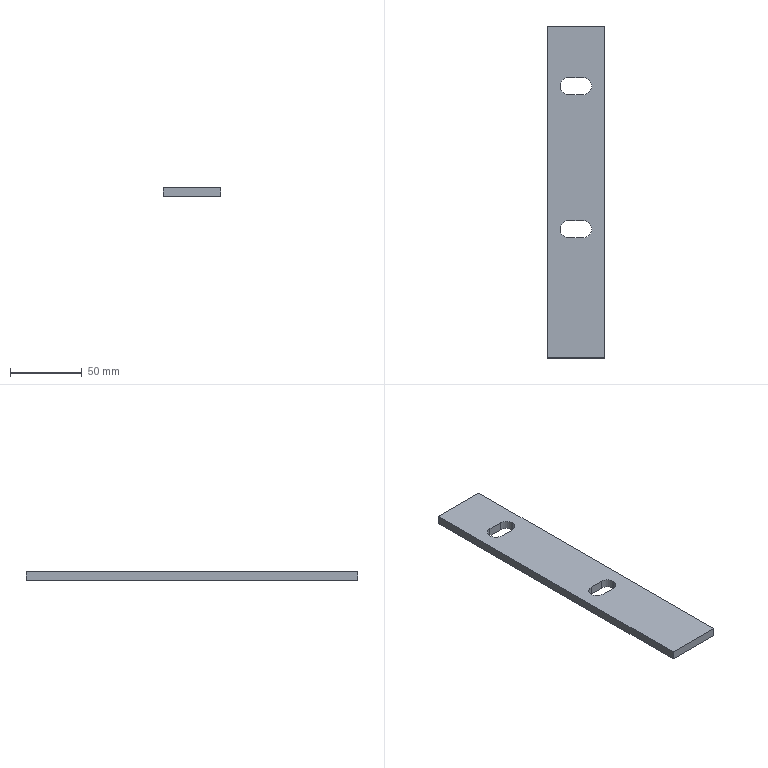Part | STEP file | 护栏连接Plate-250×125 | 1 solid | 16 faces | box 40 x 232 x 6 mm | volume 52883 mm3 | plane 10 | cylinder 6 | commonest cylinder face diameters 12 x6
STEP:
#1=CARTESIAN_POINT('',(0.,0.,0.));
#2=DIRECTION('',(0.,0.,1.));
#3=DIRECTION('',(1.,0.,0.));
#4=AXIS2_PLACEMENT_3D('',#1,#2,#3);
#5=CARTESIAN_POINT('',(5.,56.,0.));
#6=VERTEX_POINT('',#5);
#7=CARTESIAN_POINT('',(5.,56.,6.));
#8=VERTEX_POINT('',#7);
#9=CARTESIAN_POINT('',(5.,56.,6.));
#10=DIRECTION('',(0.,0.,1.));
#11=VECTOR('',#10,1.);
#12=LINE('',#9,#11);
#13=CARTESIAN_POINT('',(5.,50.,6.));
#14=DIRECTION('',(0.,0.,1.));
#15=DIRECTION('',(1.,0.,0.));
#16=AXIS2_PLACEMENT_3D('',#13,#14,#15);
#17=CYLINDRICAL_SURFACE('',#16,6.);
#18=CARTESIAN_POINT('',(1.571,0.));
#19=DIRECTION('',(0.,1.));
#20=VECTOR('',#19,1.);
#21=LINE('',#18,#20);
#22=(GEOMETRIC_REPRESENTATION_CONTEXT(2)PARAMETRIC_REPRESENTATION_CONTEXT()REPRESENTATION_CONTEXT('',''));
#23=DEFINITIONAL_REPRESENTATION('',(#21),#22);
#24=PCURVE('',#17,#23);
#25=CARTESIAN_POINT('',(-5.,56.,6.));
#26=DIRECTION('',(0.,1.,0.));
#27=DIRECTION('',(0.,0.,1.));
#28=AXIS2_PLACEMENT_3D('',#25,#26,#27);
#29=PLANE('',#28);
#30=CARTESIAN_POINT('',(0.,10.));
#31=DIRECTION('',(1.,0.));
#32=VECTOR('',#31,1.);
#33=LINE('',#30,#32);
#34=(GEOMETRIC_REPRESENTATION_CONTEXT(2)PARAMETRIC_REPRESENTATION_CONTEXT()REPRESENTATION_CONTEXT('',''));
#35=DEFINITIONAL_REPRESENTATION('',(#33),#34);
#36=PCURVE('',#29,#35);
#37=SURFACE_CURVE('',#12,(#24,#36),.PCURVE_S1.);
#38=EDGE_CURVE('',#6,#8,#37,.T.);
#39=ORIENTED_EDGE('',*,*,#38,.T.);
#40=CARTESIAN_POINT('',(11.,50.,6.));
#41=VERTEX_POINT('',#40);
#42=CARTESIAN_POINT('',(5.,50.,6.));
#43=DIRECTION('',(0.,0.,1.));
#44=DIRECTION('',(1.,0.,0.));
#45=AXIS2_PLACEMENT_3D('',#42,#43,#44);
#46=CIRCLE('',#45,6.);
#47=CARTESIAN_POINT('',(0.,0.));
#48=DIRECTION('',(1.,0.));
#49=VECTOR('',#48,1.);
#50=LINE('',#47,#49);
#51=(GEOMETRIC_REPRESENTATION_CONTEXT(2)PARAMETRIC_REPRESENTATION_CONTEXT()REPRESENTATION_CONTEXT('',''));
#52=DEFINITIONAL_REPRESENTATION('',(#50),#51);
#53=PCURVE('',#17,#52);
#54=CARTESIAN_POINT('',(0.,0.,6.));
#55=DIRECTION('',(0.,0.,1.));
#56=DIRECTION('',(1.,0.,0.));
#57=AXIS2_PLACEMENT_3D('',#54,#55,#56);
#58=PLANE('',#57);
#59=CARTESIAN_POINT('',(5.,50.));
#60=DIRECTION('',(1.,0.));
#61=AXIS2_PLACEMENT_2D('',#59,#60);
#62=CIRCLE('',#61,6.);
#63=(GEOMETRIC_REPRESENTATION_CONTEXT(2)PARAMETRIC_REPRESENTATION_CONTEXT()REPRESENTATION_CONTEXT('',''));
#64=DEFINITIONAL_REPRESENTATION('',(#62),#63);
#65=PCURVE('',#58,#64);
#66=SURFACE_CURVE('',#46,(#53,#65),.PCURVE_S1.);
#67=EDGE_CURVE('',#41,#8,#66,.T.);
#68=ORIENTED_EDGE('',*,*,#67,.F.);
#69=CARTESIAN_POINT('',(11.,50.,0.));
#70=VERTEX_POINT('',#69);
#71=CARTESIAN_POINT('',(11.,50.,6.));
#72=DIRECTION('',(0.,0.,1.));
#73=VECTOR('',#72,1.);
#74=LINE('',#71,#73);
#75=CARTESIAN_POINT('',(0.,0.));
#76=DIRECTION('',(0.,1.));
#77=VECTOR('',#76,1.);
#78=LINE('',#75,#77);
#79=(GEOMETRIC_REPRESENTATION_CONTEXT(2)PARAMETRIC_REPRESENTATION_CONTEXT()REPRESENTATION_CONTEXT('',''));
#80=DEFINITIONAL_REPRESENTATION('',(#78),#79);
#81=PCURVE('',#17,#80);
#82=CARTESIAN_POINT('',(5.,50.,6.));
#83=DIRECTION('',(0.,0.,1.));
#84=DIRECTION('',(1.,0.,0.));
#85=AXIS2_PLACEMENT_3D('',#82,#83,#84);
#86=CYLINDRICAL_SURFACE('',#85,6.);
#87=CARTESIAN_POINT('',(6.283,0.));
#88=DIRECTION('',(0.,1.));
#89=VECTOR('',#88,1.);
#90=LINE('',#87,#89);
#91=(GEOMETRIC_REPRESENTATION_CONTEXT(2)PARAMETRIC_REPRESENTATION_CONTEXT()REPRESENTATION_CONTEXT('',''));
#92=DEFINITIONAL_REPRESENTATION('',(#90),#91);
#93=PCURVE('',#86,#92);
#94=SURFACE_CURVE('',#74,(#81,#93),.PCURVE_S1.);
#95=EDGE_CURVE('',#70,#41,#94,.T.);
#96=ORIENTED_EDGE('',*,*,#95,.F.);
#97=CARTESIAN_POINT('',(5.,50.,0.));
#98=DIRECTION('',(0.,0.,1.));
#99=DIRECTION('',(1.,0.,0.));
#100=AXIS2_PLACEMENT_3D('',#97,#98,#99);
#101=CIRCLE('',#100,6.);
#102=CARTESIAN_POINT('',(0.,-6.));
#103=DIRECTION('',(1.,0.));
#104=VECTOR('',#103,1.);
#105=LINE('',#102,#104);
#106=(GEOMETRIC_REPRESENTATION_CONTEXT(2)PARAMETRIC_REPRESENTATION_CONTEXT()REPRESENTATION_CONTEXT('',''));
#107=DEFINITIONAL_REPRESENTATION('',(#105),#106);
#108=PCURVE('',#17,#107);
#109=CARTESIAN_POINT('',(0.,0.,0.));
#110=DIRECTION('',(0.,0.,1.));
#111=DIRECTION('',(1.,0.,0.));
#112=AXIS2_PLACEMENT_3D('',#109,#110,#111);
#113=PLANE('',#112);
#114=CARTESIAN_POINT('',(5.,50.));
#115=DIRECTION('',(1.,0.));
#116=AXIS2_PLACEMENT_2D('',#114,#115);
#117=CIRCLE('',#116,6.);
#118=(GEOMETRIC_REPRESENTATION_CONTEXT(2)PARAMETRIC_REPRESENTATION_CONTEXT()REPRESENTATION_CONTEXT('',''));
#119=DEFINITIONAL_REPRESENTATION('',(#117),#118);
#120=PCURVE('',#113,#119);
#121=SURFACE_CURVE('',#101,(#108,#120),.PCURVE_S1.);
#122=EDGE_CURVE('',#70,#6,#121,.T.);
#123=ORIENTED_EDGE('',*,*,#122,.T.);
#124=EDGE_LOOP('',(#39,#68,#96,#123));
#125=FACE_BOUND('',#124,.F.);
#126=ADVANCED_FACE('',(#125),#17,.F.);
#127=CARTESIAN_POINT('',(5.,-44.,0.));
#128=VERTEX_POINT('',#127);
#129=CARTESIAN_POINT('',(5.,-44.,6.));
#130=VERTEX_POINT('',#129);
#131=CARTESIAN_POINT('',(5.,-44.,6.));
#132=DIRECTION('',(0.,0.,1.));
#133=VECTOR('',#132,1.);
#134=LINE('',#131,#133);
#135=CARTESIAN_POINT('',(5.,-50.,6.));
#136=DIRECTION('',(0.,0.,1.));
#137=DIRECTION('',(1.,0.,0.));
#138=AXIS2_PLACEMENT_3D('',#135,#136,#137);
#139=CYLINDRICAL_SURFACE('',#138,6.);
#140=CARTESIAN_POINT('',(1.571,0.));
#141=DIRECTION('',(0.,1.));
#142=VECTOR('',#141,1.);
#143=LINE('',#140,#142);
#144=(GEOMETRIC_REPRESENTATION_CONTEXT(2)PARAMETRIC_REPRESENTATION_CONTEXT()REPRESENTATION_CONTEXT('',''));
#145=DEFINITIONAL_REPRESENTATION('',(#143),#144);
#146=PCURVE('',#139,#145);
#147=CARTESIAN_POINT('',(-5.,-44.,6.));
#148=DIRECTION('',(0.,1.,0.));
#149=DIRECTION('',(0.,0.,1.));
#150=AXIS2_PLACEMENT_3D('',#147,#148,#149);
#151=PLANE('',#150);
#152=CARTESIAN_POINT('',(0.,10.));
#153=DIRECTION('',(1.,0.));
#154=VECTOR('',#153,1.);
#155=LINE('',#152,#154);
#156=(GEOMETRIC_REPRESENTATION_CONTEXT(2)PARAMETRIC_REPRESENTATION_CONTEXT()REPRESENTATION_CONTEXT('',''));
#157=DEFINITIONAL_REPRESENTATION('',(#155),#156);
#158=PCURVE('',#151,#157);
#159=SURFACE_CURVE('',#134,(#146,#158),.PCURVE_S1.);
#160=EDGE_CURVE('',#128,#130,#159,.T.);
#161=ORIENTED_EDGE('',*,*,#160,.T.);
#162=CARTESIAN_POINT('',(11.,-50.,6.));
#163=VERTEX_POINT('',#162);
#164=CARTESIAN_POINT('',(5.,-50.,6.));
#165=DIRECTION('',(0.,0.,1.));
#166=DIRECTION('',(1.,0.,0.));
#167=AXIS2_PLACEMENT_3D('',#164,#165,#166);
#168=CIRCLE('',#167,6.);
#169=CARTESIAN_POINT('',(0.,0.));
#170=DIRECTION('',(1.,0.));
#171=VECTOR('',#170,1.);
#172=LINE('',#169,#171);
#173=(GEOMETRIC_REPRESENTATION_CONTEXT(2)PARAMETRIC_REPRESENTATION_CONTEXT()REPRESENTATION_CONTEXT('',''));
#174=DEFINITIONAL_REPRESENTATION('',(#172),#173);
#175=PCURVE('',#139,#174);
#176=CARTESIAN_POINT('',(5.,-50.));
#177=DIRECTION('',(1.,0.));
#178=AXIS2_PLACEMENT_2D('',#176,#177);
#179=CIRCLE('',#178,6.);
#180=(GEOMETRIC_REPRESENTATION_CONTEXT(2)PARAMETRIC_REPRESENTATION_CONTEXT()REPRESENTATION_CONTEXT('',''));
#181=DEFINITIONAL_REPRESENTATION('',(#179),#180);
#182=PCURVE('',#58,#181);
#183=SURFACE_CURVE('',#168,(#175,#182),.PCURVE_S1.);
#184=EDGE_CURVE('',#163,#130,#183,.T.);
#185=ORIENTED_EDGE('',*,*,#184,.F.);
#186=CARTESIAN_POINT('',(11.,-50.,0.));
#187=VERTEX_POINT('',#186);
#188=CARTESIAN_POINT('',(11.,-50.,6.));
#189=DIRECTION('',(0.,0.,1.));
#190=VECTOR('',#189,1.);
#191=LINE('',#188,#190);
#192=CARTESIAN_POINT('',(0.,0.));
#193=DIRECTION('',(0.,1.));
#194=VECTOR('',#193,1.);
#195=LINE('',#192,#194);
#196=(GEOMETRIC_REPRESENTATION_CONTEXT(2)PARAMETRIC_REPRESENTATION_CONTEXT()REPRESENTATION_CONTEXT('',''));
#197=DEFINITIONAL_REPRESENTATION('',(#195),#196);
#198=PCURVE('',#139,#197);
#199=CARTESIAN_POINT('',(5.,-50.,6.));
#200=DIRECTION('',(0.,0.,1.));
#201=DIRECTION('',(1.,0.,0.));
#202=AXIS2_PLACEMENT_3D('',#199,#200,#201);
#203=CYLINDRICAL_SURFACE('',#202,6.);
#204=CARTESIAN_POINT('',(6.283,0.));
#205=DIRECTION('',(0.,1.));
#206=VECTOR('',#205,1.);
#207=LINE('',#204,#206);
#208=(GEOMETRIC_REPRESENTATION_CONTEXT(2)PARAMETRIC_REPRESENTATION_CONTEXT()REPRESENTATION_CONTEXT('',''));
#209=DEFINITIONAL_REPRESENTATION('',(#207),#208);
#210=PCURVE('',#203,#209);
#211=SURFACE_CURVE('',#191,(#198,#210),.PCURVE_S1.);
#212=EDGE_CURVE('',#187,#163,#211,.T.);
#213=ORIENTED_EDGE('',*,*,#212,.F.);
#214=CARTESIAN_POINT('',(5.,-50.,0.));
#215=DIRECTION('',(0.,0.,1.));
#216=DIRECTION('',(1.,0.,0.));
#217=AXIS2_PLACEMENT_3D('',#214,#215,#216);
#218=CIRCLE('',#217,6.);
#219=CARTESIAN_POINT('',(0.,-6.));
#220=DIRECTION('',(1.,0.));
#221=VECTOR('',#220,1.);
#222=LINE('',#219,#221);
#223=(GEOMETRIC_REPRESENTATION_CONTEXT(2)PARAMETRIC_REPRESENTATION_CONTEXT()REPRESENTATION_CONTEXT('',''));
#224=DEFINITIONAL_REPRESENTATION('',(#222),#223);
#225=PCURVE('',#139,#224);
#226=CARTESIAN_POINT('',(5.,-50.));
#227=DIRECTION('',(1.,0.));
#228=AXIS2_PLACEMENT_2D('',#226,#227);
#229=CIRCLE('',#228,6.);
#230=(GEOMETRIC_REPRESENTATION_CONTEXT(2)PARAMETRIC_REPRESENTATION_CONTEXT()REPRESENTATION_CONTEXT('',''));
#231=DEFINITIONAL_REPRESENTATION('',(#229),#230);
#232=PCURVE('',#113,#231);
#233=SURFACE_CURVE('',#218,(#225,#232),.PCURVE_S1.);
#234=EDGE_CURVE('',#187,#128,#233,.T.);
#235=ORIENTED_EDGE('',*,*,#234,.T.);
#236=EDGE_LOOP('',(#161,#185,#213,#235));
#237=FACE_BOUND('',#236,.F.);
#238=ADVANCED_FACE('',(#237),#139,.F.);
#239=CARTESIAN_POINT('',(20.,-140.,0.));
#240=VERTEX_POINT('',#239);
#241=CARTESIAN_POINT('',(20.,92.,0.));
#242=VERTEX_POINT('',#241);
#243=CARTESIAN_POINT('',(20.,92.,0.));
#244=DIRECTION('',(0.,1.,0.));
#245=VECTOR('',#244,1.);
#246=LINE('',#243,#245);
#247=CARTESIAN_POINT('',(20.,92.,6.));
#248=DIRECTION('',(-1.,0.,0.));
#249=DIRECTION('',(0.,-1.,0.));
#250=AXIS2_PLACEMENT_3D('',#247,#248,#249);
#251=PLANE('',#250);
#252=CARTESIAN_POINT('',(0.,-6.));
#253=DIRECTION('',(-1.,0.));
#254=VECTOR('',#253,1.);
#255=LINE('',#252,#254);
#256=(GEOMETRIC_REPRESENTATION_CONTEXT(2)PARAMETRIC_REPRESENTATION_CONTEXT()REPRESENTATION_CONTEXT('',''));
#257=DEFINITIONAL_REPRESENTATION('',(#255),#256);
#258=PCURVE('',#251,#257);
#259=CARTESIAN_POINT('',(20.,92.));
#260=DIRECTION('',(0.,1.));
#261=VECTOR('',#260,1.);
#262=LINE('',#259,#261);
#263=(GEOMETRIC_REPRESENTATION_CONTEXT(2)PARAMETRIC_REPRESENTATION_CONTEXT()REPRESENTATION_CONTEXT('',''));
#264=DEFINITIONAL_REPRESENTATION('',(#262),#263);
#265=PCURVE('',#113,#264);
#266=SURFACE_CURVE('',#246,(#258,#265),.PCURVE_S1.);
#267=EDGE_CURVE('',#240,#242,#266,.T.);
#268=ORIENTED_EDGE('',*,*,#267,.T.);
#269=CARTESIAN_POINT('',(20.,92.,6.));
#270=VERTEX_POINT('',#269);
#271=CARTESIAN_POINT('',(20.,92.,6.));
#272=DIRECTION('',(0.,0.,-1.));
#273=VECTOR('',#272,1.);
#274=LINE('',#271,#273);
#275=CARTESIAN_POINT('',(0.,0.));
#276=DIRECTION('',(0.,-1.));
#277=VECTOR('',#276,1.);
#278=LINE('',#275,#277);
#279=(GEOMETRIC_REPRESENTATION_CONTEXT(2)PARAMETRIC_REPRESENTATION_CONTEXT()REPRESENTATION_CONTEXT('',''));
#280=DEFINITIONAL_REPRESENTATION('',(#278),#279);
#281=PCURVE('',#251,#280);
#282=CARTESIAN_POINT('',(-20.,92.,6.));
#283=DIRECTION('',(0.,-1.,0.));
#284=DIRECTION('',(0.,0.,-1.));
#285=AXIS2_PLACEMENT_3D('',#282,#283,#284);
#286=PLANE('',#285);
#287=CARTESIAN_POINT('',(0.,40.));
#288=DIRECTION('',(1.,0.));
#289=VECTOR('',#288,1.);
#290=LINE('',#287,#289);
#291=(GEOMETRIC_REPRESENTATION_CONTEXT(2)PARAMETRIC_REPRESENTATION_CONTEXT()REPRESENTATION_CONTEXT('',''));
#292=DEFINITIONAL_REPRESENTATION('',(#290),#291);
#293=PCURVE('',#286,#292);
#294=SURFACE_CURVE('',#274,(#281,#293),.PCURVE_S1.);
#295=EDGE_CURVE('',#270,#242,#294,.T.);
#296=ORIENTED_EDGE('',*,*,#295,.F.);
#297=CARTESIAN_POINT('',(20.,-140.,6.));
#298=VERTEX_POINT('',#297);
#299=CARTESIAN_POINT('',(20.,92.,6.));
#300=DIRECTION('',(0.,1.,0.));
#301=VECTOR('',#300,1.);
#302=LINE('',#299,#301);
#303=CARTESIAN_POINT('',(0.,0.));
#304=DIRECTION('',(-1.,0.));
#305=VECTOR('',#304,1.);
#306=LINE('',#303,#305);
#307=(GEOMETRIC_REPRESENTATION_CONTEXT(2)PARAMETRIC_REPRESENTATION_CONTEXT()REPRESENTATION_CONTEXT('',''));
#308=DEFINITIONAL_REPRESENTATION('',(#306),#307);
#309=PCURVE('',#251,#308);
#310=CARTESIAN_POINT('',(20.,92.));
#311=DIRECTION('',(0.,1.));
#312=VECTOR('',#311,1.);
#313=LINE('',#310,#312);
#314=(GEOMETRIC_REPRESENTATION_CONTEXT(2)PARAMETRIC_REPRESENTATION_CONTEXT()REPRESENTATION_CONTEXT('',''));
#315=DEFINITIONAL_REPRESENTATION('',(#313),#314);
#316=PCURVE('',#58,#315);
#317=SURFACE_CURVE('',#302,(#309,#316),.PCURVE_S1.);
#318=EDGE_CURVE('',#298,#270,#317,.T.);
#319=ORIENTED_EDGE('',*,*,#318,.F.);
#320=CARTESIAN_POINT('',(20.,-140.,6.));
#321=DIRECTION('',(0.,0.,-1.));
#322=VECTOR('',#321,1.);
#323=LINE('',#320,#322);
#324=CARTESIAN_POINT('',(232.,0.));
#325=DIRECTION('',(0.,-1.));
#326=VECTOR('',#325,1.);
#327=LINE('',#324,#326);
#328=(GEOMETRIC_REPRESENTATION_CONTEXT(2)PARAMETRIC_REPRESENTATION_CONTEXT()REPRESENTATION_CONTEXT('',''));
#329=DEFINITIONAL_REPRESENTATION('',(#327),#328);
#330=PCURVE('',#251,#329);
#331=CARTESIAN_POINT('',(-20.,-140.,6.));
#332=DIRECTION('',(0.,1.,0.));
#333=DIRECTION('',(0.,0.,1.));
#334=AXIS2_PLACEMENT_3D('',#331,#332,#333);
#335=PLANE('',#334);
#336=CARTESIAN_POINT('',(0.,40.));
#337=DIRECTION('',(-1.,0.));
#338=VECTOR('',#337,1.);
#339=LINE('',#336,#338);
#340=(GEOMETRIC_REPRESENTATION_CONTEXT(2)PARAMETRIC_REPRESENTATION_CONTEXT()REPRESENTATION_CONTEXT('',''));
#341=DEFINITIONAL_REPRESENTATION('',(#339),#340);
#342=PCURVE('',#335,#341);
#343=SURFACE_CURVE('',#323,(#330,#342),.PCURVE_S1.);
#344=EDGE_CURVE('',#298,#240,#343,.T.);
#345=ORIENTED_EDGE('',*,*,#344,.T.);
#346=EDGE_LOOP('',(#268,#296,#319,#345));
#347=FACE_BOUND('',#346,.T.);
#348=ADVANCED_FACE('',(#347),#251,.F.);
#349=CARTESIAN_POINT('',(-20.,92.,0.));
#350=VERTEX_POINT('',#349);
#351=CARTESIAN_POINT('',(-20.,92.,0.));
#352=DIRECTION('',(-1.,0.,0.));
#353=VECTOR('',#352,1.);
#354=LINE('',#351,#353);
#355=CARTESIAN_POINT('',(6.,0.));
#356=DIRECTION('',(0.,-1.));
#357=VECTOR('',#356,1.);
#358=LINE('',#355,#357);
#359=(GEOMETRIC_REPRESENTATION_CONTEXT(2)PARAMETRIC_REPRESENTATION_CONTEXT()REPRESENTATION_CONTEXT('',''));
#360=DEFINITIONAL_REPRESENTATION('',(#358),#359);
#361=PCURVE('',#286,#360);
#362=CARTESIAN_POINT('',(-20.,92.));
#363=DIRECTION('',(-1.,0.));
#364=VECTOR('',#363,1.);
#365=LINE('',#362,#364);
#366=(GEOMETRIC_REPRESENTATION_CONTEXT(2)PARAMETRIC_REPRESENTATION_CONTEXT()REPRESENTATION_CONTEXT('',''));
#367=DEFINITIONAL_REPRESENTATION('',(#365),#366);
#368=PCURVE('',#113,#367);
#369=SURFACE_CURVE('',#354,(#361,#368),.PCURVE_S1.);
#370=EDGE_CURVE('',#242,#350,#369,.T.);
#371=ORIENTED_EDGE('',*,*,#370,.T.);
#372=CARTESIAN_POINT('',(-20.,92.,6.));
#373=VERTEX_POINT('',#372);
#374=CARTESIAN_POINT('',(-20.,92.,6.));
#375=DIRECTION('',(0.,0.,-1.));
#376=VECTOR('',#375,1.);
#377=LINE('',#374,#376);
#378=CARTESIAN_POINT('',(0.,0.));
#379=DIRECTION('',(1.,0.));
#380=VECTOR('',#379,1.);
#381=LINE('',#378,#380);
#382=(GEOMETRIC_REPRESENTATION_CONTEXT(2)PARAMETRIC_REPRESENTATION_CONTEXT()REPRESENTATION_CONTEXT('',''));
#383=DEFINITIONAL_REPRESENTATION('',(#381),#382);
#384=PCURVE('',#286,#383);
#385=CARTESIAN_POINT('',(-20.,92.,6.));
#386=DIRECTION('',(1.,0.,0.));
#387=DIRECTION('',(0.,1.,0.));
#388=AXIS2_PLACEMENT_3D('',#385,#386,#387);
#389=PLANE('',#388);
#390=CARTESIAN_POINT('',(0.,0.));
#391=DIRECTION('',(0.,-1.));
#392=VECTOR('',#391,1.);
#393=LINE('',#390,#392);
#394=(GEOMETRIC_REPRESENTATION_CONTEXT(2)PARAMETRIC_REPRESENTATION_CONTEXT()REPRESENTATION_CONTEXT('',''));
#395=DEFINITIONAL_REPRESENTATION('',(#393),#394);
#396=PCURVE('',#389,#395);
#397=SURFACE_CURVE('',#377,(#384,#396),.PCURVE_S1.);
#398=EDGE_CURVE('',#373,#350,#397,.T.);
#399=ORIENTED_EDGE('',*,*,#398,.F.);
#400=CARTESIAN_POINT('',(-20.,92.,6.));
#401=DIRECTION('',(-1.,0.,0.));
#402=VECTOR('',#401,1.);
#403=LINE('',#400,#402);
#404=CARTESIAN_POINT('',(0.,0.));
#405=DIRECTION('',(0.,-1.));
#406=VECTOR('',#405,1.);
#407=LINE('',#404,#406);
#408=(GEOMETRIC_REPRESENTATION_CONTEXT(2)PARAMETRIC_REPRESENTATION_CONTEXT()REPRESENTATION_CONTEXT('',''));
#409=DEFINITIONAL_REPRESENTATION('',(#407),#408);
#410=PCURVE('',#286,#409);
#411=CARTESIAN_POINT('',(-20.,92.));
#412=DIRECTION('',(-1.,0.));
#413=VECTOR('',#412,1.);
#414=LINE('',#411,#413);
#415=(GEOMETRIC_REPRESENTATION_CONTEXT(2)PARAMETRIC_REPRESENTATION_CONTEXT()REPRESENTATION_CONTEXT('',''));
#416=DEFINITIONAL_REPRESENTATION('',(#414),#415);
#417=PCURVE('',#58,#416);
#418=SURFACE_CURVE('',#403,(#410,#417),.PCURVE_S1.);
#419=EDGE_CURVE('',#270,#373,#418,.T.);
#420=ORIENTED_EDGE('',*,*,#419,.F.);
#421=ORIENTED_EDGE('',*,*,#295,.T.);
#422=EDGE_LOOP('',(#371,#399,#420,#421));
#423=FACE_BOUND('',#422,.T.);
#424=ADVANCED_FACE('',(#423),#286,.F.);
#425=CARTESIAN_POINT('',(-20.,-140.,0.));
#426=VERTEX_POINT('',#425);
#427=CARTESIAN_POINT('',(-20.,92.,0.));
#428=DIRECTION('',(0.,-1.,0.));
#429=VECTOR('',#428,1.);
#430=LINE('',#427,#429);
#431=CARTESIAN_POINT('',(0.,-6.));
#432=DIRECTION('',(-1.,0.));
#433=VECTOR('',#432,1.);
#434=LINE('',#431,#433);
#435=(GEOMETRIC_REPRESENTATION_CONTEXT(2)PARAMETRIC_REPRESENTATION_CONTEXT()REPRESENTATION_CONTEXT('',''));
#436=DEFINITIONAL_REPRESENTATION('',(#434),#435);
#437=PCURVE('',#389,#436);
#438=CARTESIAN_POINT('',(-20.,92.));
#439=DIRECTION('',(0.,-1.));
#440=VECTOR('',#439,1.);
#441=LINE('',#438,#440);
#442=(GEOMETRIC_REPRESENTATION_CONTEXT(2)PARAMETRIC_REPRESENTATION_CONTEXT()REPRESENTATION_CONTEXT('',''));
#443=DEFINITIONAL_REPRESENTATION('',(#441),#442);
#444=PCURVE('',#113,#443);
#445=SURFACE_CURVE('',#430,(#437,#444),.PCURVE_S1.);
#446=EDGE_CURVE('',#350,#426,#445,.T.);
#447=ORIENTED_EDGE('',*,*,#446,.T.);
#448=CARTESIAN_POINT('',(-20.,-140.,6.));
#449=VERTEX_POINT('',#448);
#450=CARTESIAN_POINT('',(-20.,-140.,6.));
#451=DIRECTION('',(0.,0.,-1.));
#452=VECTOR('',#451,1.);
#453=LINE('',#450,#452);
#454=CARTESIAN_POINT('',(-232.,0.));
#455=DIRECTION('',(0.,-1.));
#456=VECTOR('',#455,1.);
#457=LINE('',#454,#456);
#458=(GEOMETRIC_REPRESENTATION_CONTEXT(2)PARAMETRIC_REPRESENTATION_CONTEXT()REPRESENTATION_CONTEXT('',''));
#459=DEFINITIONAL_REPRESENTATION('',(#457),#458);
#460=PCURVE('',#389,#459);
#461=CARTESIAN_POINT('',(0.,0.));
#462=DIRECTION('',(-1.,0.));
#463=VECTOR('',#462,1.);
#464=LINE('',#461,#463);
#465=(GEOMETRIC_REPRESENTATION_CONTEXT(2)PARAMETRIC_REPRESENTATION_CONTEXT()REPRESENTATION_CONTEXT('',''));
#466=DEFINITIONAL_REPRESENTATION('',(#464),#465);
#467=PCURVE('',#335,#466);
#468=SURFACE_CURVE('',#453,(#460,#467),.PCURVE_S1.);
#469=EDGE_CURVE('',#449,#426,#468,.T.);
#470=ORIENTED_EDGE('',*,*,#469,.F.);
#471=CARTESIAN_POINT('',(-20.,92.,6.));
#472=DIRECTION('',(0.,-1.,0.));
#473=VECTOR('',#472,1.);
#474=LINE('',#471,#473);
#475=CARTESIAN_POINT('',(0.,0.));
#476=DIRECTION('',(-1.,0.));
#477=VECTOR('',#476,1.);
#478=LINE('',#475,#477);
#479=(GEOMETRIC_REPRESENTATION_CONTEXT(2)PARAMETRIC_REPRESENTATION_CONTEXT()REPRESENTATION_CONTEXT('',''));
#480=DEFINITIONAL_REPRESENTATION('',(#478),#479);
#481=PCURVE('',#389,#480);
#482=CARTESIAN_POINT('',(-20.,92.));
#483=DIRECTION('',(0.,-1.));
#484=VECTOR('',#483,1.);
#485=LINE('',#482,#484);
#486=(GEOMETRIC_REPRESENTATION_CONTEXT(2)PARAMETRIC_REPRESENTATION_CONTEXT()REPRESENTATION_CONTEXT('',''));
#487=DEFINITIONAL_REPRESENTATION('',(#485),#486);
#488=PCURVE('',#58,#487);
#489=SURFACE_CURVE('',#474,(#481,#488),.PCURVE_S1.);
#490=EDGE_CURVE('',#373,#449,#489,.T.);
#491=ORIENTED_EDGE('',*,*,#490,.F.);
#492=ORIENTED_EDGE('',*,*,#398,.T.);
#493=EDGE_LOOP('',(#447,#470,#491,#492));
#494=FACE_BOUND('',#493,.T.);
#495=ADVANCED_FACE('',(#494),#389,.F.);
#496=CARTESIAN_POINT('',(-20.,-140.,0.));
#497=DIRECTION('',(1.,0.,0.));
#498=VECTOR('',#497,1.);
#499=LINE('',#496,#498);
#500=CARTESIAN_POINT('',(-6.,0.));
#501=DIRECTION('',(0.,1.));
#502=VECTOR('',#501,1.);
#503=LINE('',#500,#502);
#504=(GEOMETRIC_REPRESENTATION_CONTEXT(2)PARAMETRIC_REPRESENTATION_CONTEXT()REPRESENTATION_CONTEXT('',''));
#505=DEFINITIONAL_REPRESENTATION('',(#503),#504);
#506=PCURVE('',#335,#505);
#507=CARTESIAN_POINT('',(-20.,-140.));
#508=DIRECTION('',(1.,0.));
#509=VECTOR('',#508,1.);
#510=LINE('',#507,#509);
#511=(GEOMETRIC_REPRESENTATION_CONTEXT(2)PARAMETRIC_REPRESENTATION_CONTEXT()REPRESENTATION_CONTEXT('',''));
#512=DEFINITIONAL_REPRESENTATION('',(#510),#511);
#513=PCURVE('',#113,#512);
#514=SURFACE_CURVE('',#499,(#506,#513),.PCURVE_S1.);
#515=EDGE_CURVE('',#426,#240,#514,.T.);
#516=ORIENTED_EDGE('',*,*,#515,.T.);
#517=ORIENTED_EDGE('',*,*,#344,.F.);
#518=CARTESIAN_POINT('',(-20.,-140.,6.));
#519=DIRECTION('',(1.,0.,0.));
#520=VECTOR('',#519,1.);
#521=LINE('',#518,#520);
#522=CARTESIAN_POINT('',(0.,0.));
#523=DIRECTION('',(0.,1.));
#524=VECTOR('',#523,1.);
#525=LINE('',#522,#524);
#526=(GEOMETRIC_REPRESENTATION_CONTEXT(2)PARAMETRIC_REPRESENTATION_CONTEXT()REPRESENTATION_CONTEXT('',''));
#527=DEFINITIONAL_REPRESENTATION('',(#525),#526);
#528=PCURVE('',#335,#527);
#529=CARTESIAN_POINT('',(-20.,-140.));
#530=DIRECTION('',(1.,0.));
#531=VECTOR('',#530,1.);
#532=LINE('',#529,#531);
#533=(GEOMETRIC_REPRESENTATION_CONTEXT(2)PARAMETRIC_REPRESENTATION_CONTEXT()REPRESENTATION_CONTEXT('',''));
#534=DEFINITIONAL_REPRESENTATION('',(#532),#533);
#535=PCURVE('',#58,#534);
#536=SURFACE_CURVE('',#521,(#528,#535),.PCURVE_S1.);
#537=EDGE_CURVE('',#449,#298,#536,.T.);
#538=ORIENTED_EDGE('',*,*,#537,.F.);
#539=ORIENTED_EDGE('',*,*,#469,.T.);
#540=EDGE_LOOP('',(#516,#517,#538,#539));
#541=FACE_BOUND('',#540,.T.);
#542=ADVANCED_FACE('',(#541),#335,.F.);
#543=CARTESIAN_POINT('',(-5.,56.,6.));
#544=VERTEX_POINT('',#543);
#545=CARTESIAN_POINT('',(-5.,56.,6.));
#546=DIRECTION('',(1.,0.,0.));
#547=VECTOR('',#546,1.);
#548=LINE('',#545,#547);
#549=CARTESIAN_POINT('',(-5.,56.));
#550=DIRECTION('',(1.,0.));
#551=VECTOR('',#550,1.);
#552=LINE('',#549,#551);
#553=(GEOMETRIC_REPRESENTATION_CONTEXT(2)PARAMETRIC_REPRESENTATION_CONTEXT()REPRESENTATION_CONTEXT('',''));
#554=DEFINITIONAL_REPRESENTATION('',(#552),#553);
#555=PCURVE('',#58,#554);
#556=CARTESIAN_POINT('',(0.,0.));
#557=DIRECTION('',(0.,1.));
#558=VECTOR('',#557,1.);
#559=LINE('',#556,#558);
#560=(GEOMETRIC_REPRESENTATION_CONTEXT(2)PARAMETRIC_REPRESENTATION_CONTEXT()REPRESENTATION_CONTEXT('',''));
#561=DEFINITIONAL_REPRESENTATION('',(#559),#560);
#562=PCURVE('',#29,#561);
#563=SURFACE_CURVE('',#548,(#555,#562),.PCURVE_S1.);
#564=EDGE_CURVE('',#544,#8,#563,.T.);
#565=ORIENTED_EDGE('',*,*,#564,.T.);
#566=ORIENTED_EDGE('',*,*,#67,.F.);
#567=CARTESIAN_POINT('',(5.,44.,6.));
#568=VERTEX_POINT('',#567);
#569=CARTESIAN_POINT('',(5.,50.,6.));
#570=DIRECTION('',(0.,0.,1.));
#571=DIRECTION('',(1.,0.,0.));
#572=AXIS2_PLACEMENT_3D('',#569,#570,#571);
#573=CIRCLE('',#572,6.);
#574=CARTESIAN_POINT('',(5.,50.));
#575=DIRECTION('',(1.,0.));
#576=AXIS2_PLACEMENT_2D('',#574,#575);
#577=CIRCLE('',#576,6.);
#578=(GEOMETRIC_REPRESENTATION_CONTEXT(2)PARAMETRIC_REPRESENTATION_CONTEXT()REPRESENTATION_CONTEXT('',''));
#579=DEFINITIONAL_REPRESENTATION('',(#577),#578);
#580=PCURVE('',#58,#579);
#581=CARTESIAN_POINT('',(0.,0.));
#582=DIRECTION('',(1.,0.));
#583=VECTOR('',#582,1.);
#584=LINE('',#581,#583);
#585=(GEOMETRIC_REPRESENTATION_CONTEXT(2)PARAMETRIC_REPRESENTATION_CONTEXT()REPRESENTATION_CONTEXT('',''));
#586=DEFINITIONAL_REPRESENTATION('',(#584),#585);
#587=PCURVE('',#86,#586);
#588=SURFACE_CURVE('',#573,(#580,#587),.PCURVE_S1.);
#589=EDGE_CURVE('',#568,#41,#588,.T.);
#590=ORIENTED_EDGE('',*,*,#589,.F.);
#591=CARTESIAN_POINT('',(-5.,44.,6.));
#592=VERTEX_POINT('',#591);
#593=CARTESIAN_POINT('',(-5.,44.,6.));
#594=DIRECTION('',(1.,0.,0.));
#595=VECTOR('',#594,1.);
#596=LINE('',#593,#595);
#597=CARTESIAN_POINT('',(-5.,44.));
#598=DIRECTION('',(1.,0.));
#599=VECTOR('',#598,1.);
#600=LINE('',#597,#599);
#601=(GEOMETRIC_REPRESENTATION_CONTEXT(2)PARAMETRIC_REPRESENTATION_CONTEXT()REPRESENTATION_CONTEXT('',''));
#602=DEFINITIONAL_REPRESENTATION('',(#600),#601);
#603=PCURVE('',#58,#602);
#604=CARTESIAN_POINT('',(-5.,44.,6.));
#605=DIRECTION('',(0.,-1.,0.));
#606=DIRECTION('',(0.,0.,-1.));
#607=AXIS2_PLACEMENT_3D('',#604,#605,#606);
#608=PLANE('',#607);
#609=CARTESIAN_POINT('',(0.,0.));
#610=DIRECTION('',(0.,1.));
#611=VECTOR('',#610,1.);
#612=LINE('',#609,#611);
#613=(GEOMETRIC_REPRESENTATION_CONTEXT(2)PARAMETRIC_REPRESENTATION_CONTEXT()REPRESENTATION_CONTEXT('',''));
#614=DEFINITIONAL_REPRESENTATION('',(#612),#613);
#615=PCURVE('',#608,#614);
#616=SURFACE_CURVE('',#596,(#603,#615),.PCURVE_S1.);
#617=EDGE_CURVE('',#592,#568,#616,.T.);
#618=ORIENTED_EDGE('',*,*,#617,.F.);
#619=CARTESIAN_POINT('',(-5.,50.,6.));
#620=DIRECTION('',(0.,0.,1.));
#621=DIRECTION('',(1.,0.,0.));
#622=AXIS2_PLACEMENT_3D('',#619,#620,#621);
#623=CIRCLE('',#622,6.);
#624=CARTESIAN_POINT('',(-5.,50.));
#625=DIRECTION('',(1.,0.));
#626=AXIS2_PLACEMENT_2D('',#624,#625);
#627=CIRCLE('',#626,6.);
#628=(GEOMETRIC_REPRESENTATION_CONTEXT(2)PARAMETRIC_REPRESENTATION_CONTEXT()REPRESENTATION_CONTEXT('',''));
#629=DEFINITIONAL_REPRESENTATION('',(#627),#628);
#630=PCURVE('',#58,#629);
#631=CARTESIAN_POINT('',(-5.,50.,6.));
#632=DIRECTION('',(0.,0.,1.));
#633=DIRECTION('',(1.,0.,0.));
#634=AXIS2_PLACEMENT_3D('',#631,#632,#633);
#635=CYLINDRICAL_SURFACE('',#634,6.);
#636=CARTESIAN_POINT('',(0.,0.));
#637=DIRECTION('',(1.,0.));
#638=VECTOR('',#637,1.);
#639=LINE('',#636,#638);
#640=(GEOMETRIC_REPRESENTATION_CONTEXT(2)PARAMETRIC_REPRESENTATION_CONTEXT()REPRESENTATION_CONTEXT('',''));
#641=DEFINITIONAL_REPRESENTATION('',(#639),#640);
#642=PCURVE('',#635,#641);
#643=SURFACE_CURVE('',#623,(#630,#642),.PCURVE_S1.);
#644=EDGE_CURVE('',#544,#592,#643,.T.);
#645=ORIENTED_EDGE('',*,*,#644,.F.);
#646=EDGE_LOOP('',(#565,#566,#590,#618,#645));
#647=FACE_BOUND('',#646,.T.);
#648=CARTESIAN_POINT('',(5.,-56.,6.));
#649=VERTEX_POINT('',#648);
#650=CARTESIAN_POINT('',(5.,-50.,6.));
#651=DIRECTION('',(0.,0.,1.));
#652=DIRECTION('',(1.,0.,0.));
#653=AXIS2_PLACEMENT_3D('',#650,#651,#652);
#654=CIRCLE('',#653,6.);
#655=CARTESIAN_POINT('',(5.,-50.));
#656=DIRECTION('',(1.,0.));
#657=AXIS2_PLACEMENT_2D('',#655,#656);
#658=CIRCLE('',#657,6.);
#659=(GEOMETRIC_REPRESENTATION_CONTEXT(2)PARAMETRIC_REPRESENTATION_CONTEXT()REPRESENTATION_CONTEXT('',''));
#660=DEFINITIONAL_REPRESENTATION('',(#658),#659);
#661=PCURVE('',#58,#660);
#662=CARTESIAN_POINT('',(0.,0.));
#663=DIRECTION('',(1.,0.));
#664=VECTOR('',#663,1.);
#665=LINE('',#662,#664);
#666=(GEOMETRIC_REPRESENTATION_CONTEXT(2)PARAMETRIC_REPRESENTATION_CONTEXT()REPRESENTATION_CONTEXT('',''));
#667=DEFINITIONAL_REPRESENTATION('',(#665),#666);
#668=PCURVE('',#203,#667);
#669=SURFACE_CURVE('',#654,(#661,#668),.PCURVE_S1.);
#670=EDGE_CURVE('',#649,#163,#669,.T.);
#671=ORIENTED_EDGE('',*,*,#670,.F.);
#672=CARTESIAN_POINT('',(-5.,-56.,6.));
#673=VERTEX_POINT('',#672);
#674=CARTESIAN_POINT('',(-5.,-56.,6.));
#675=DIRECTION('',(1.,0.,0.));
#676=VECTOR('',#675,1.);
#677=LINE('',#674,#676);
#678=CARTESIAN_POINT('',(-5.,-56.));
#679=DIRECTION('',(1.,0.));
#680=VECTOR('',#679,1.);
#681=LINE('',#678,#680);
#682=(GEOMETRIC_REPRESENTATION_CONTEXT(2)PARAMETRIC_REPRESENTATION_CONTEXT()REPRESENTATION_CONTEXT('',''));
#683=DEFINITIONAL_REPRESENTATION('',(#681),#682);
#684=PCURVE('',#58,#683);
#685=CARTESIAN_POINT('',(-5.,-56.,6.));
#686=DIRECTION('',(0.,-1.,0.));
#687=DIRECTION('',(0.,0.,-1.));
#688=AXIS2_PLACEMENT_3D('',#685,#686,#687);
#689=PLANE('',#688);
#690=CARTESIAN_POINT('',(0.,0.));
#691=DIRECTION('',(0.,1.));
#692=VECTOR('',#691,1.);
#693=LINE('',#690,#692);
#694=(GEOMETRIC_REPRESENTATION_CONTEXT(2)PARAMETRIC_REPRESENTATION_CONTEXT()REPRESENTATION_CONTEXT('',''));
#695=DEFINITIONAL_REPRESENTATION('',(#693),#694);
#696=PCURVE('',#689,#695);
#697=SURFACE_CURVE('',#677,(#684,#696),.PCURVE_S1.);
#698=EDGE_CURVE('',#673,#649,#697,.T.);
#699=ORIENTED_EDGE('',*,*,#698,.F.);
#700=CARTESIAN_POINT('',(-5.,-44.,6.));
#701=VERTEX_POINT('',#700);
#702=CARTESIAN_POINT('',(-5.,-50.,6.));
#703=DIRECTION('',(0.,0.,1.));
#704=DIRECTION('',(1.,0.,0.));
#705=AXIS2_PLACEMENT_3D('',#702,#703,#704);
#706=CIRCLE('',#705,6.);
#707=CARTESIAN_POINT('',(-5.,-50.));
#708=DIRECTION('',(1.,0.));
#709=AXIS2_PLACEMENT_2D('',#707,#708);
#710=CIRCLE('',#709,6.);
#711=(GEOMETRIC_REPRESENTATION_CONTEXT(2)PARAMETRIC_REPRESENTATION_CONTEXT()REPRESENTATION_CONTEXT('',''));
#712=DEFINITIONAL_REPRESENTATION('',(#710),#711);
#713=PCURVE('',#58,#712);
#714=CARTESIAN_POINT('',(-5.,-50.,6.));
#715=DIRECTION('',(0.,0.,1.));
#716=DIRECTION('',(1.,0.,0.));
#717=AXIS2_PLACEMENT_3D('',#714,#715,#716);
#718=CYLINDRICAL_SURFACE('',#717,6.);
#719=CARTESIAN_POINT('',(0.,0.));
#720=DIRECTION('',(1.,0.));
#721=VECTOR('',#720,1.);
#722=LINE('',#719,#721);
#723=(GEOMETRIC_REPRESENTATION_CONTEXT(2)PARAMETRIC_REPRESENTATION_CONTEXT()REPRESENTATION_CONTEXT('',''));
#724=DEFINITIONAL_REPRESENTATION('',(#722),#723);
#725=PCURVE('',#718,#724);
#726=SURFACE_CURVE('',#706,(#713,#725),.PCURVE_S1.);
#727=EDGE_CURVE('',#701,#673,#726,.T.);
#728=ORIENTED_EDGE('',*,*,#727,.F.);
#729=CARTESIAN_POINT('',(-5.,-44.,6.));
#730=DIRECTION('',(1.,0.,0.));
#731=VECTOR('',#730,1.);
#732=LINE('',#729,#731);
#733=CARTESIAN_POINT('',(-5.,-44.));
#734=DIRECTION('',(1.,0.));
#735=VECTOR('',#734,1.);
#736=LINE('',#733,#735);
#737=(GEOMETRIC_REPRESENTATION_CONTEXT(2)PARAMETRIC_REPRESENTATION_CONTEXT()REPRESENTATION_CONTEXT('',''));
#738=DEFINITIONAL_REPRESENTATION('',(#736),#737);
#739=PCURVE('',#58,#738);
#740=CARTESIAN_POINT('',(0.,0.));
#741=DIRECTION('',(0.,1.));
#742=VECTOR('',#741,1.);
#743=LINE('',#740,#742);
#744=(GEOMETRIC_REPRESENTATION_CONTEXT(2)PARAMETRIC_REPRESENTATION_CONTEXT()REPRESENTATION_CONTEXT('',''));
#745=DEFINITIONAL_REPRESENTATION('',(#743),#744);
#746=PCURVE('',#151,#745);
#747=SURFACE_CURVE('',#732,(#739,#746),.PCURVE_S1.);
#748=EDGE_CURVE('',#701,#130,#747,.T.);
#749=ORIENTED_EDGE('',*,*,#748,.T.);
#750=ORIENTED_EDGE('',*,*,#184,.F.);
#751=EDGE_LOOP('',(#671,#699,#728,#749,#750));
#752=FACE_BOUND('',#751,.T.);
#753=ORIENTED_EDGE('',*,*,#318,.T.);
#754=ORIENTED_EDGE('',*,*,#419,.T.);
#755=ORIENTED_EDGE('',*,*,#490,.T.);
#756=ORIENTED_EDGE('',*,*,#537,.T.);
#757=EDGE_LOOP('',(#753,#754,#755,#756));
#758=FACE_BOUND('',#757,.T.);
#759=ADVANCED_FACE('',(#647,#752,#758),#58,.T.);
#760=CARTESIAN_POINT('',(-5.,44.,0.));
#761=VERTEX_POINT('',#760);
#762=CARTESIAN_POINT('',(5.,44.,0.));
#763=VERTEX_POINT('',#762);
#764=CARTESIAN_POINT('',(-5.,44.,0.));
#765=DIRECTION('',(1.,0.,0.));
#766=VECTOR('',#765,1.);
#767=LINE('',#764,#766);
#768=CARTESIAN_POINT('',(-5.,44.));
#769=DIRECTION('',(1.,0.));
#770=VECTOR('',#769,1.);
#771=LINE('',#768,#770);
#772=(GEOMETRIC_REPRESENTATION_CONTEXT(2)PARAMETRIC_REPRESENTATION_CONTEXT()REPRESENTATION_CONTEXT('',''));
#773=DEFINITIONAL_REPRESENTATION('',(#771),#772);
#774=PCURVE('',#113,#773);
#775=CARTESIAN_POINT('',(6.,0.));
#776=DIRECTION('',(0.,1.));
#777=VECTOR('',#776,1.);
#778=LINE('',#775,#777);
#779=(GEOMETRIC_REPRESENTATION_CONTEXT(2)PARAMETRIC_REPRESENTATION_CONTEXT()REPRESENTATION_CONTEXT('',''));
#780=DEFINITIONAL_REPRESENTATION('',(#778),#779);
#781=PCURVE('',#608,#780);
#782=SURFACE_CURVE('',#767,(#774,#781),.PCURVE_S1.);
#783=EDGE_CURVE('',#761,#763,#782,.T.);
#784=ORIENTED_EDGE('',*,*,#783,.T.);
#785=CARTESIAN_POINT('',(5.,50.,0.));
#786=DIRECTION('',(0.,0.,1.));
#787=DIRECTION('',(1.,0.,0.));
#788=AXIS2_PLACEMENT_3D('',#785,#786,#787);
#789=CIRCLE('',#788,6.);
#790=CARTESIAN_POINT('',(5.,50.));
#791=DIRECTION('',(1.,0.));
#792=AXIS2_PLACEMENT_2D('',#790,#791);
#793=CIRCLE('',#792,6.);
#794=(GEOMETRIC_REPRESENTATION_CONTEXT(2)PARAMETRIC_REPRESENTATION_CONTEXT()REPRESENTATION_CONTEXT('',''));
#795=DEFINITIONAL_REPRESENTATION('',(#793),#794);
#796=PCURVE('',#113,#795);
#797=CARTESIAN_POINT('',(0.,-6.));
#798=DIRECTION('',(1.,0.));
#799=VECTOR('',#798,1.);
#800=LINE('',#797,#799);
#801=(GEOMETRIC_REPRESENTATION_CONTEXT(2)PARAMETRIC_REPRESENTATION_CONTEXT()REPRESENTATION_CONTEXT('',''));
#802=DEFINITIONAL_REPRESENTATION('',(#800),#801);
#803=PCURVE('',#86,#802);
#804=SURFACE_CURVE('',#789,(#796,#803),.PCURVE_S1.);
#805=EDGE_CURVE('',#763,#70,#804,.T.);
#806=ORIENTED_EDGE('',*,*,#805,.T.);
#807=ORIENTED_EDGE('',*,*,#122,.T.);
#808=CARTESIAN_POINT('',(-5.,56.,0.));
#809=VERTEX_POINT('',#808);
#810=CARTESIAN_POINT('',(-5.,56.,0.));
#811=DIRECTION('',(1.,0.,0.));
#812=VECTOR('',#811,1.);
#813=LINE('',#810,#812);
#814=CARTESIAN_POINT('',(-5.,56.));
#815=DIRECTION('',(1.,0.));
#816=VECTOR('',#815,1.);
#817=LINE('',#814,#816);
#818=(GEOMETRIC_REPRESENTATION_CONTEXT(2)PARAMETRIC_REPRESENTATION_CONTEXT()REPRESENTATION_CONTEXT('',''));
#819=DEFINITIONAL_REPRESENTATION('',(#817),#818);
#820=PCURVE('',#113,#819);
#821=CARTESIAN_POINT('',(-6.,0.));
#822=DIRECTION('',(0.,1.));
#823=VECTOR('',#822,1.);
#824=LINE('',#821,#823);
#825=(GEOMETRIC_REPRESENTATION_CONTEXT(2)PARAMETRIC_REPRESENTATION_CONTEXT()REPRESENTATION_CONTEXT('',''));
#826=DEFINITIONAL_REPRESENTATION('',(#824),#825);
#827=PCURVE('',#29,#826);
#828=SURFACE_CURVE('',#813,(#820,#827),.PCURVE_S1.);
#829=EDGE_CURVE('',#809,#6,#828,.T.);
#830=ORIENTED_EDGE('',*,*,#829,.F.);
#831=CARTESIAN_POINT('',(-5.,50.,0.));
#832=DIRECTION('',(0.,0.,1.));
#833=DIRECTION('',(1.,0.,0.));
#834=AXIS2_PLACEMENT_3D('',#831,#832,#833);
#835=CIRCLE('',#834,6.);
#836=CARTESIAN_POINT('',(-5.,50.));
#837=DIRECTION('',(1.,0.));
#838=AXIS2_PLACEMENT_2D('',#836,#837);
#839=CIRCLE('',#838,6.);
#840=(GEOMETRIC_REPRESENTATION_CONTEXT(2)PARAMETRIC_REPRESENTATION_CONTEXT()REPRESENTATION_CONTEXT('',''));
#841=DEFINITIONAL_REPRESENTATION('',(#839),#840);
#842=PCURVE('',#113,#841);
#843=CARTESIAN_POINT('',(0.,-6.));
#844=DIRECTION('',(1.,0.));
#845=VECTOR('',#844,1.);
#846=LINE('',#843,#845);
#847=(GEOMETRIC_REPRESENTATION_CONTEXT(2)PARAMETRIC_REPRESENTATION_CONTEXT()REPRESENTATION_CONTEXT('',''));
#848=DEFINITIONAL_REPRESENTATION('',(#846),#847);
#849=PCURVE('',#635,#848);
#850=SURFACE_CURVE('',#835,(#842,#849),.PCURVE_S1.);
#851=EDGE_CURVE('',#809,#761,#850,.T.);
#852=ORIENTED_EDGE('',*,*,#851,.T.);
#853=EDGE_LOOP('',(#784,#806,#807,#830,#852));
#854=FACE_BOUND('',#853,.T.);
#855=CARTESIAN_POINT('',(5.,-56.,0.));
#856=VERTEX_POINT('',#855);
#857=CARTESIAN_POINT('',(5.,-50.,0.));
#858=DIRECTION('',(0.,0.,1.));
#859=DIRECTION('',(1.,0.,0.));
#860=AXIS2_PLACEMENT_3D('',#857,#858,#859);
#861=CIRCLE('',#860,6.);
#862=CARTESIAN_POINT('',(5.,-50.));
#863=DIRECTION('',(1.,0.));
#864=AXIS2_PLACEMENT_2D('',#862,#863);
#865=CIRCLE('',#864,6.);
#866=(GEOMETRIC_REPRESENTATION_CONTEXT(2)PARAMETRIC_REPRESENTATION_CONTEXT()REPRESENTATION_CONTEXT('',''));
#867=DEFINITIONAL_REPRESENTATION('',(#865),#866);
#868=PCURVE('',#113,#867);
#869=CARTESIAN_POINT('',(0.,-6.));
#870=DIRECTION('',(1.,0.));
#871=VECTOR('',#870,1.);
#872=LINE('',#869,#871);
#873=(GEOMETRIC_REPRESENTATION_CONTEXT(2)PARAMETRIC_REPRESENTATION_CONTEXT()REPRESENTATION_CONTEXT('',''));
#874=DEFINITIONAL_REPRESENTATION('',(#872),#873);
#875=PCURVE('',#203,#874);
#876=SURFACE_CURVE('',#861,(#868,#875),.PCURVE_S1.);
#877=EDGE_CURVE('',#856,#187,#876,.T.);
#878=ORIENTED_EDGE('',*,*,#877,.T.);
#879=ORIENTED_EDGE('',*,*,#234,.T.);
#880=CARTESIAN_POINT('',(-5.,-44.,0.));
#881=VERTEX_POINT('',#880);
#882=CARTESIAN_POINT('',(-5.,-44.,0.));
#883=DIRECTION('',(1.,0.,0.));
#884=VECTOR('',#883,1.);
#885=LINE('',#882,#884);
#886=CARTESIAN_POINT('',(-5.,-44.));
#887=DIRECTION('',(1.,0.));
#888=VECTOR('',#887,1.);
#889=LINE('',#886,#888);
#890=(GEOMETRIC_REPRESENTATION_CONTEXT(2)PARAMETRIC_REPRESENTATION_CONTEXT()REPRESENTATION_CONTEXT('',''));
#891=DEFINITIONAL_REPRESENTATION('',(#889),#890);
#892=PCURVE('',#113,#891);
#893=CARTESIAN_POINT('',(-6.,0.));
#894=DIRECTION('',(0.,1.));
#895=VECTOR('',#894,1.);
#896=LINE('',#893,#895);
#897=(GEOMETRIC_REPRESENTATION_CONTEXT(2)PARAMETRIC_REPRESENTATION_CONTEXT()REPRESENTATION_CONTEXT('',''));
#898=DEFINITIONAL_REPRESENTATION('',(#896),#897);
#899=PCURVE('',#151,#898);
#900=SURFACE_CURVE('',#885,(#892,#899),.PCURVE_S1.);
#901=EDGE_CURVE('',#881,#128,#900,.T.);
#902=ORIENTED_EDGE('',*,*,#901,.F.);
#903=CARTESIAN_POINT('',(-5.,-56.,0.));
#904=VERTEX_POINT('',#903);
#905=CARTESIAN_POINT('',(-5.,-50.,0.));
#906=DIRECTION('',(0.,0.,1.));
#907=DIRECTION('',(1.,0.,0.));
#908=AXIS2_PLACEMENT_3D('',#905,#906,#907);
#909=CIRCLE('',#908,6.);
#910=CARTESIAN_POINT('',(-5.,-50.));
#911=DIRECTION('',(1.,0.));
#912=AXIS2_PLACEMENT_2D('',#910,#911);
#913=CIRCLE('',#912,6.);
#914=(GEOMETRIC_REPRESENTATION_CONTEXT(2)PARAMETRIC_REPRESENTATION_CONTEXT()REPRESENTATION_CONTEXT('',''));
#915=DEFINITIONAL_REPRESENTATION('',(#913),#914);
#916=PCURVE('',#113,#915);
#917=CARTESIAN_POINT('',(0.,-6.));
#918=DIRECTION('',(1.,0.));
#919=VECTOR('',#918,1.);
#920=LINE('',#917,#919);
#921=(GEOMETRIC_REPRESENTATION_CONTEXT(2)PARAMETRIC_REPRESENTATION_CONTEXT()REPRESENTATION_CONTEXT('',''));
#922=DEFINITIONAL_REPRESENTATION('',(#920),#921);
#923=PCURVE('',#718,#922);
#924=SURFACE_CURVE('',#909,(#916,#923),.PCURVE_S1.);
#925=EDGE_CURVE('',#881,#904,#924,.T.);
#926=ORIENTED_EDGE('',*,*,#925,.T.);
#927=CARTESIAN_POINT('',(-5.,-56.,0.));
#928=DIRECTION('',(1.,0.,0.));
#929=VECTOR('',#928,1.);
#930=LINE('',#927,#929);
#931=CARTESIAN_POINT('',(-5.,-56.));
#932=DIRECTION('',(1.,0.));
#933=VECTOR('',#932,1.);
#934=LINE('',#931,#933);
#935=(GEOMETRIC_REPRESENTATION_CONTEXT(2)PARAMETRIC_REPRESENTATION_CONTEXT()REPRESENTATION_CONTEXT('',''));
#936=DEFINITIONAL_REPRESENTATION('',(#934),#935);
#937=PCURVE('',#113,#936);
#938=CARTESIAN_POINT('',(6.,0.));
#939=DIRECTION('',(0.,1.));
#940=VECTOR('',#939,1.);
#941=LINE('',#938,#940);
#942=(GEOMETRIC_REPRESENTATION_CONTEXT(2)PARAMETRIC_REPRESENTATION_CONTEXT()REPRESENTATION_CONTEXT('',''));
#943=DEFINITIONAL_REPRESENTATION('',(#941),#942);
#944=PCURVE('',#689,#943);
#945=SURFACE_CURVE('',#930,(#937,#944),.PCURVE_S1.);
#946=EDGE_CURVE('',#904,#856,#945,.T.);
#947=ORIENTED_EDGE('',*,*,#946,.T.);
#948=EDGE_LOOP('',(#878,#879,#902,#926,#947));
#949=FACE_BOUND('',#948,.T.);
#950=ORIENTED_EDGE('',*,*,#267,.F.);
#951=ORIENTED_EDGE('',*,*,#515,.F.);
#952=ORIENTED_EDGE('',*,*,#446,.F.);
#953=ORIENTED_EDGE('',*,*,#370,.F.);
#954=EDGE_LOOP('',(#950,#951,#952,#953));
#955=FACE_BOUND('',#954,.T.);
#956=ADVANCED_FACE('',(#854,#949,#955),#113,.F.);
#957=ORIENTED_EDGE('',*,*,#670,.F.);
#958=CARTESIAN_POINT('',(5.,-56.,6.));
#959=DIRECTION('',(0.,0.,-1.));
#960=VECTOR('',#959,1.);
#961=LINE('',#958,#960);
#962=CARTESIAN_POINT('',(4.712,0.));
#963=DIRECTION('',(0.,-1.));
#964=VECTOR('',#963,1.);
#965=LINE('',#962,#964);
#966=(GEOMETRIC_REPRESENTATION_CONTEXT(2)PARAMETRIC_REPRESENTATION_CONTEXT()REPRESENTATION_CONTEXT('',''));
#967=DEFINITIONAL_REPRESENTATION('',(#965),#966);
#968=PCURVE('',#203,#967);
#969=CARTESIAN_POINT('',(0.,10.));
#970=DIRECTION('',(1.,0.));
#971=VECTOR('',#970,1.);
#972=LINE('',#969,#971);
#973=(GEOMETRIC_REPRESENTATION_CONTEXT(2)PARAMETRIC_REPRESENTATION_CONTEXT()REPRESENTATION_CONTEXT('',''));
#974=DEFINITIONAL_REPRESENTATION('',(#972),#973);
#975=PCURVE('',#689,#974);
#976=SURFACE_CURVE('',#961,(#968,#975),.PCURVE_S1.);
#977=EDGE_CURVE('',#649,#856,#976,.T.);
#978=ORIENTED_EDGE('',*,*,#977,.T.);
#979=ORIENTED_EDGE('',*,*,#877,.T.);
#980=ORIENTED_EDGE('',*,*,#212,.T.);
#981=EDGE_LOOP('',(#957,#978,#979,#980));
#982=FACE_BOUND('',#981,.F.);
#983=ADVANCED_FACE('',(#982),#203,.F.);
#984=CARTESIAN_POINT('',(-5.,-44.,6.));
#985=DIRECTION('',(0.,0.,-1.));
#986=VECTOR('',#985,1.);
#987=LINE('',#984,#986);
#988=CARTESIAN_POINT('',(1.571,0.));
#989=DIRECTION('',(0.,-1.));
#990=VECTOR('',#989,1.);
#991=LINE('',#988,#990);
#992=(GEOMETRIC_REPRESENTATION_CONTEXT(2)PARAMETRIC_REPRESENTATION_CONTEXT()REPRESENTATION_CONTEXT('',''));
#993=DEFINITIONAL_REPRESENTATION('',(#991),#992);
#994=PCURVE('',#718,#993);
#995=CARTESIAN_POINT('',(0.,0.));
#996=DIRECTION('',(-1.,0.));
#997=VECTOR('',#996,1.);
#998=LINE('',#995,#997);
#999=(GEOMETRIC_REPRESENTATION_CONTEXT(2)PARAMETRIC_REPRESENTATION_CONTEXT()REPRESENTATION_CONTEXT('',''));
#1000=DEFINITIONAL_REPRESENTATION('',(#998),#999);
#1001=PCURVE('',#151,#1000);
#1002=SURFACE_CURVE('',#987,(#994,#1001),.PCURVE_S1.);
#1003=EDGE_CURVE('',#701,#881,#1002,.T.);
#1004=ORIENTED_EDGE('',*,*,#1003,.T.);
#1005=ORIENTED_EDGE('',*,*,#925,.T.);
#1006=CARTESIAN_POINT('',(-5.,-56.,6.));
#1007=DIRECTION('',(0.,0.,1.));
#1008=VECTOR('',#1007,1.);
#1009=LINE('',#1006,#1008);
#1010=CARTESIAN_POINT('',(4.712,0.));
#1011=DIRECTION('',(0.,1.));
#1012=VECTOR('',#1011,1.);
#1013=LINE('',#1010,#1012);
#1014=(GEOMETRIC_REPRESENTATION_CONTEXT(2)PARAMETRIC_REPRESENTATION_CONTEXT()REPRESENTATION_CONTEXT('',''));
#1015=DEFINITIONAL_REPRESENTATION('',(#1013),#1014);
#1016=PCURVE('',#718,#1015);
#1017=CARTESIAN_POINT('',(0.,0.));
#1018=DIRECTION('',(-1.,0.));
#1019=VECTOR('',#1018,1.);
#1020=LINE('',#1017,#1019);
#1021=(GEOMETRIC_REPRESENTATION_CONTEXT(2)PARAMETRIC_REPRESENTATION_CONTEXT()REPRESENTATION_CONTEXT('',''));
#1022=DEFINITIONAL_REPRESENTATION('',(#1020),#1021);
#1023=PCURVE('',#689,#1022);
#1024=SURFACE_CURVE('',#1009,(#1016,#1023),.PCURVE_S1.);
#1025=EDGE_CURVE('',#904,#673,#1024,.T.);
#1026=ORIENTED_EDGE('',*,*,#1025,.T.);
#1027=ORIENTED_EDGE('',*,*,#727,.F.);
#1028=EDGE_LOOP('',(#1004,#1005,#1026,#1027));
#1029=FACE_BOUND('',#1028,.F.);
#1030=ADVANCED_FACE('',(#1029),#718,.F.);
#1031=ORIENTED_EDGE('',*,*,#160,.T.);
#1032=ORIENTED_EDGE('',*,*,#748,.F.);
#1033=ORIENTED_EDGE('',*,*,#1003,.T.);
#1034=ORIENTED_EDGE('',*,*,#901,.T.);
#1035=EDGE_LOOP('',(#1031,#1032,#1033,#1034));
#1036=FACE_BOUND('',#1035,.T.);
#1037=ADVANCED_FACE('',(#1036),#151,.F.);
#1038=ORIENTED_EDGE('',*,*,#977,.T.);
#1039=ORIENTED_EDGE('',*,*,#946,.F.);
#1040=ORIENTED_EDGE('',*,*,#1025,.T.);
#1041=ORIENTED_EDGE('',*,*,#698,.T.);
#1042=EDGE_LOOP('',(#1038,#1039,#1040,#1041));
#1043=FACE_BOUND('',#1042,.T.);
#1044=ADVANCED_FACE('',(#1043),#689,.F.);
#1045=ORIENTED_EDGE('',*,*,#589,.F.);
#1046=CARTESIAN_POINT('',(5.,44.,6.));
#1047=DIRECTION('',(0.,0.,-1.));
#1048=VECTOR('',#1047,1.);
#1049=LINE('',#1046,#1048);
#1050=CARTESIAN_POINT('',(4.712,0.));
#1051=DIRECTION('',(0.,-1.));
#1052=VECTOR('',#1051,1.);
#1053=LINE('',#1050,#1052);
#1054=(GEOMETRIC_REPRESENTATION_CONTEXT(2)PARAMETRIC_REPRESENTATION_CONTEXT()REPRESENTATION_CONTEXT('',''));
#1055=DEFINITIONAL_REPRESENTATION('',(#1053),#1054);
#1056=PCURVE('',#86,#1055);
#1057=CARTESIAN_POINT('',(0.,10.));
#1058=DIRECTION('',(1.,0.));
#1059=VECTOR('',#1058,1.);
#1060=LINE('',#1057,#1059);
#1061=(GEOMETRIC_REPRESENTATION_CONTEXT(2)PARAMETRIC_REPRESENTATION_CONTEXT()REPRESENTATION_CONTEXT('',''));
#1062=DEFINITIONAL_REPRESENTATION('',(#1060),#1061);
#1063=PCURVE('',#608,#1062);
#1064=SURFACE_CURVE('',#1049,(#1056,#1063),.PCURVE_S1.);
#1065=EDGE_CURVE('',#568,#763,#1064,.T.);
#1066=ORIENTED_EDGE('',*,*,#1065,.T.);
#1067=ORIENTED_EDGE('',*,*,#805,.T.);
#1068=ORIENTED_EDGE('',*,*,#95,.T.);
#1069=EDGE_LOOP('',(#1045,#1066,#1067,#1068));
#1070=FACE_BOUND('',#1069,.F.);
#1071=ADVANCED_FACE('',(#1070),#86,.F.);
#1072=CARTESIAN_POINT('',(-5.,56.,6.));
#1073=DIRECTION('',(0.,0.,-1.));
#1074=VECTOR('',#1073,1.);
#1075=LINE('',#1072,#1074);
#1076=CARTESIAN_POINT('',(1.571,0.));
#1077=DIRECTION('',(0.,-1.));
#1078=VECTOR('',#1077,1.);
#1079=LINE('',#1076,#1078);
#1080=(GEOMETRIC_REPRESENTATION_CONTEXT(2)PARAMETRIC_REPRESENTATION_CONTEXT()REPRESENTATION_CONTEXT('',''));
#1081=DEFINITIONAL_REPRESENTATION('',(#1079),#1080);
#1082=PCURVE('',#635,#1081);
#1083=CARTESIAN_POINT('',(0.,0.));
#1084=DIRECTION('',(-1.,0.));
#1085=VECTOR('',#1084,1.);
#1086=LINE('',#1083,#1085);
#1087=(GEOMETRIC_REPRESENTATION_CONTEXT(2)PARAMETRIC_REPRESENTATION_CONTEXT()REPRESENTATION_CONTEXT('',''));
#1088=DEFINITIONAL_REPRESENTATION('',(#1086),#1087);
#1089=PCURVE('',#29,#1088);
#1090=SURFACE_CURVE('',#1075,(#1082,#1089),.PCURVE_S1.);
#1091=EDGE_CURVE('',#544,#809,#1090,.T.);
#1092=ORIENTED_EDGE('',*,*,#1091,.T.);
#1093=ORIENTED_EDGE('',*,*,#851,.T.);
#1094=CARTESIAN_POINT('',(-5.,44.,6.));
#1095=DIRECTION('',(0.,0.,1.));
#1096=VECTOR('',#1095,1.);
#1097=LINE('',#1094,#1096);
#1098=CARTESIAN_POINT('',(4.712,0.));
#1099=DIRECTION('',(0.,1.));
#1100=VECTOR('',#1099,1.);
#1101=LINE('',#1098,#1100);
#1102=(GEOMETRIC_REPRESENTATION_CONTEXT(2)PARAMETRIC_REPRESENTATION_CONTEXT()REPRESENTATION_CONTEXT('',''));
#1103=DEFINITIONAL_REPRESENTATION('',(#1101),#1102);
#1104=PCURVE('',#635,#1103);
#1105=CARTESIAN_POINT('',(0.,0.));
#1106=DIRECTION('',(-1.,0.));
#1107=VECTOR('',#1106,1.);
#1108=LINE('',#1105,#1107);
#1109=(GEOMETRIC_REPRESENTATION_CONTEXT(2)PARAMETRIC_REPRESENTATION_CONTEXT()REPRESENTATION_CONTEXT('',''));
#1110=DEFINITIONAL_REPRESENTATION('',(#1108),#1109);
#1111=PCURVE('',#608,#1110);
#1112=SURFACE_CURVE('',#1097,(#1104,#1111),.PCURVE_S1.);
#1113=EDGE_CURVE('',#761,#592,#1112,.T.);
#1114=ORIENTED_EDGE('',*,*,#1113,.T.);
#1115=ORIENTED_EDGE('',*,*,#644,.F.);
#1116=EDGE_LOOP('',(#1092,#1093,#1114,#1115));
#1117=FACE_BOUND('',#1116,.F.);
#1118=ADVANCED_FACE('',(#1117),#635,.F.);
#1119=ORIENTED_EDGE('',*,*,#38,.T.);
#1120=ORIENTED_EDGE('',*,*,#564,.F.);
#1121=ORIENTED_EDGE('',*,*,#1091,.T.);
#1122=ORIENTED_EDGE('',*,*,#829,.T.);
#1123=EDGE_LOOP('',(#1119,#1120,#1121,#1122));
#1124=FACE_BOUND('',#1123,.T.);
#1125=ADVANCED_FACE('',(#1124),#29,.F.);
#1126=ORIENTED_EDGE('',*,*,#1065,.T.);
#1127=ORIENTED_EDGE('',*,*,#783,.F.);
#1128=ORIENTED_EDGE('',*,*,#1113,.T.);
#1129=ORIENTED_EDGE('',*,*,#617,.T.);
#1130=EDGE_LOOP('',(#1126,#1127,#1128,#1129));
#1131=FACE_BOUND('',#1130,.T.);
#1132=ADVANCED_FACE('',(#1131),#608,.F.);
#1133=CLOSED_SHELL('',(#126,#238,#348,#424,#495,#542,#759,#956,#983,#1030,#1037,#1044,#1071,#1118,#1125,#1132));
#1134=MANIFOLD_SOLID_BREP('',#1133);
#1135=(LENGTH_UNIT()NAMED_UNIT(*)SI_UNIT(.MILLI.,.METRE.));
#1136=UNCERTAINTY_MEASURE_WITH_UNIT(LENGTH_MEASURE(0.0000001),#1135,'','');
#1137=(NAMED_UNIT(*)PLANE_ANGLE_UNIT()SI_UNIT($,.RADIAN.));
#1138=(NAMED_UNIT(*)SI_UNIT($,.STERADIAN.)SOLID_ANGLE_UNIT());
#1139=(GEOMETRIC_REPRESENTATION_CONTEXT(3)GLOBAL_UNCERTAINTY_ASSIGNED_CONTEXT((#1136))GLOBAL_UNIT_ASSIGNED_CONTEXT((#1135,#1137,#1138))REPRESENTATION_CONTEXT('',''));
#1140=ADVANCED_BREP_SHAPE_REPRESENTATION('',(#4,#1134),#1139);